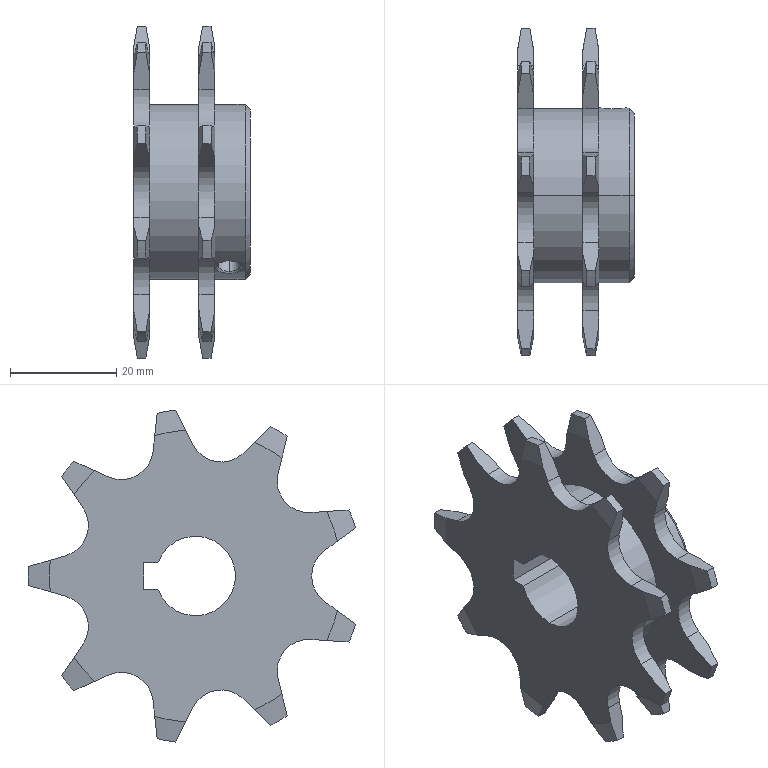Part | STEP file | WESP3-9-N15 double-speed chain; wheel | 1 solid | 135 faces | box 22 x 61.668 x 62.567 mm | volume 21694 mm3 | cylinder 48 | plane 45 | cone 42 | commonest cylinder face diameters 11.91 x18 63 x18 4.134 x4 33 x4 15 x3 20 x1